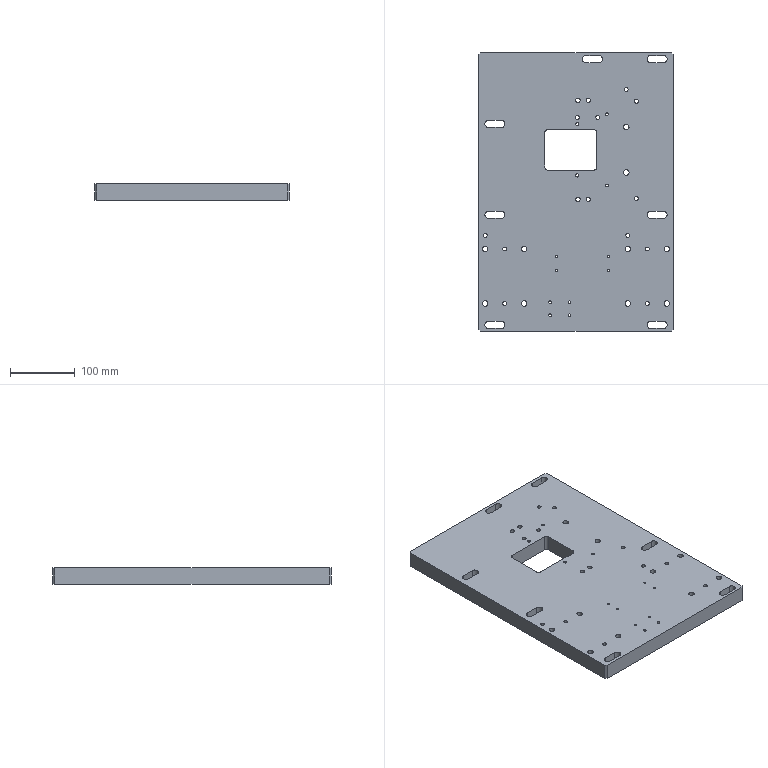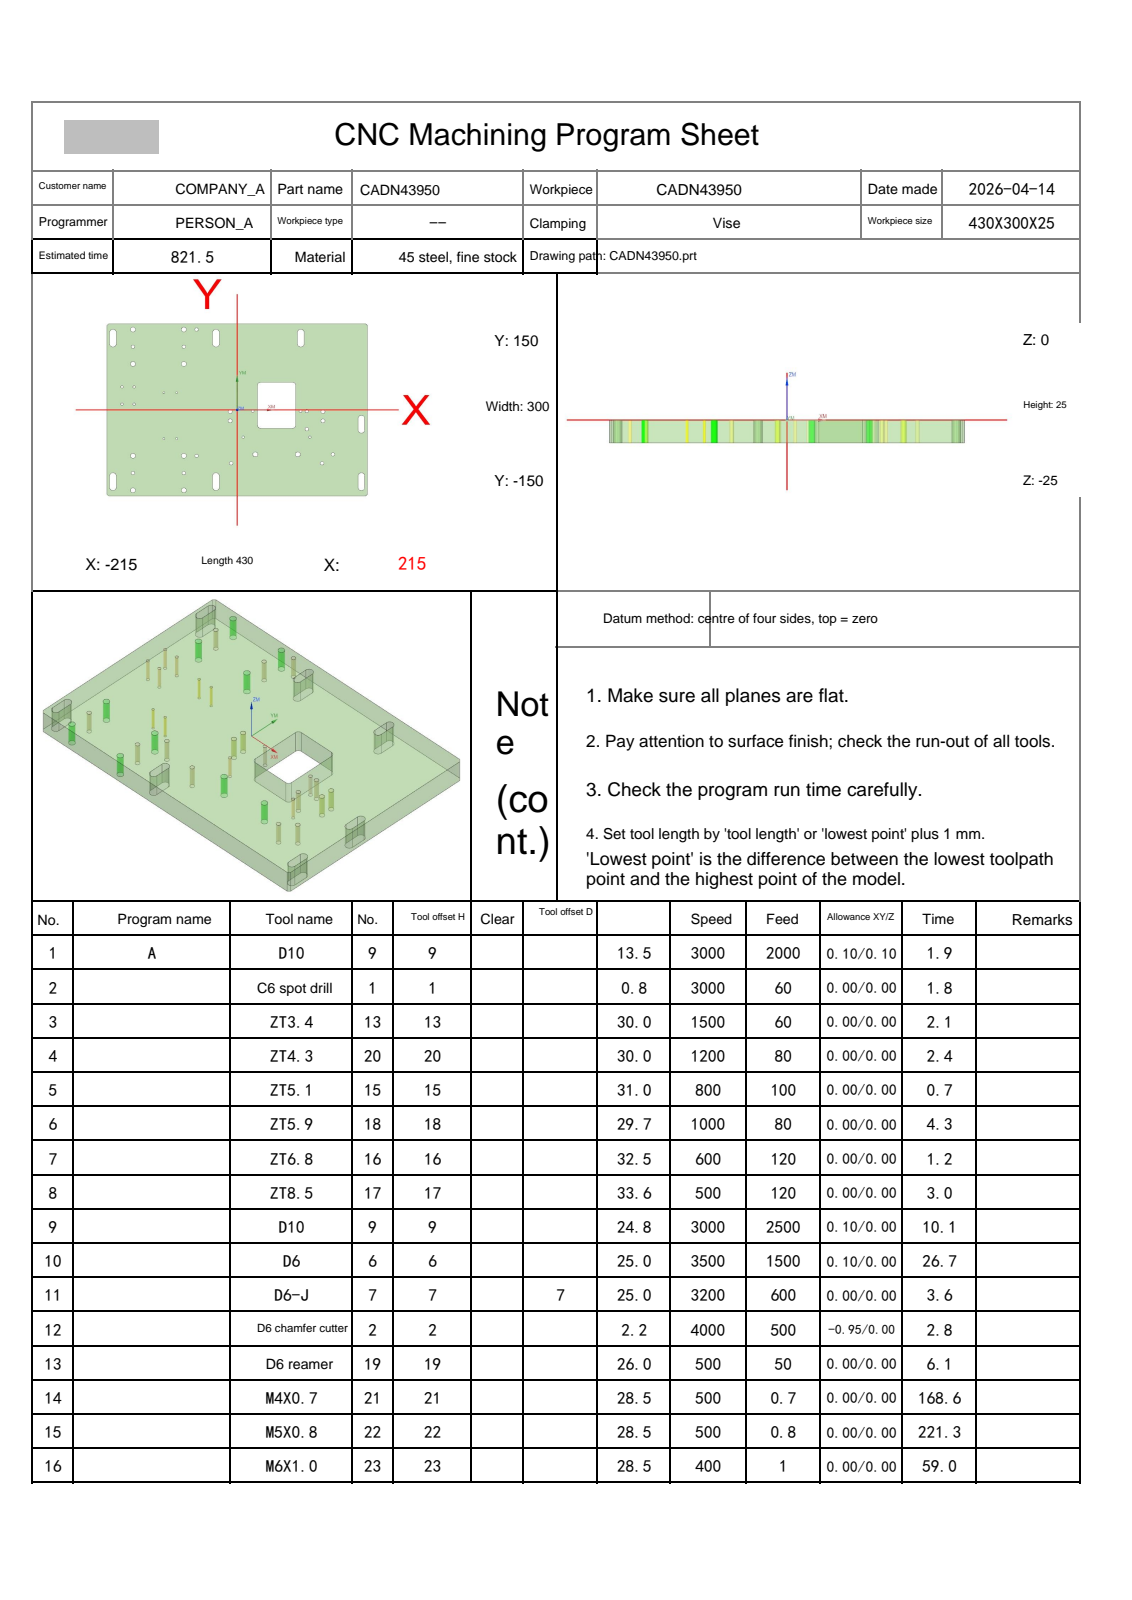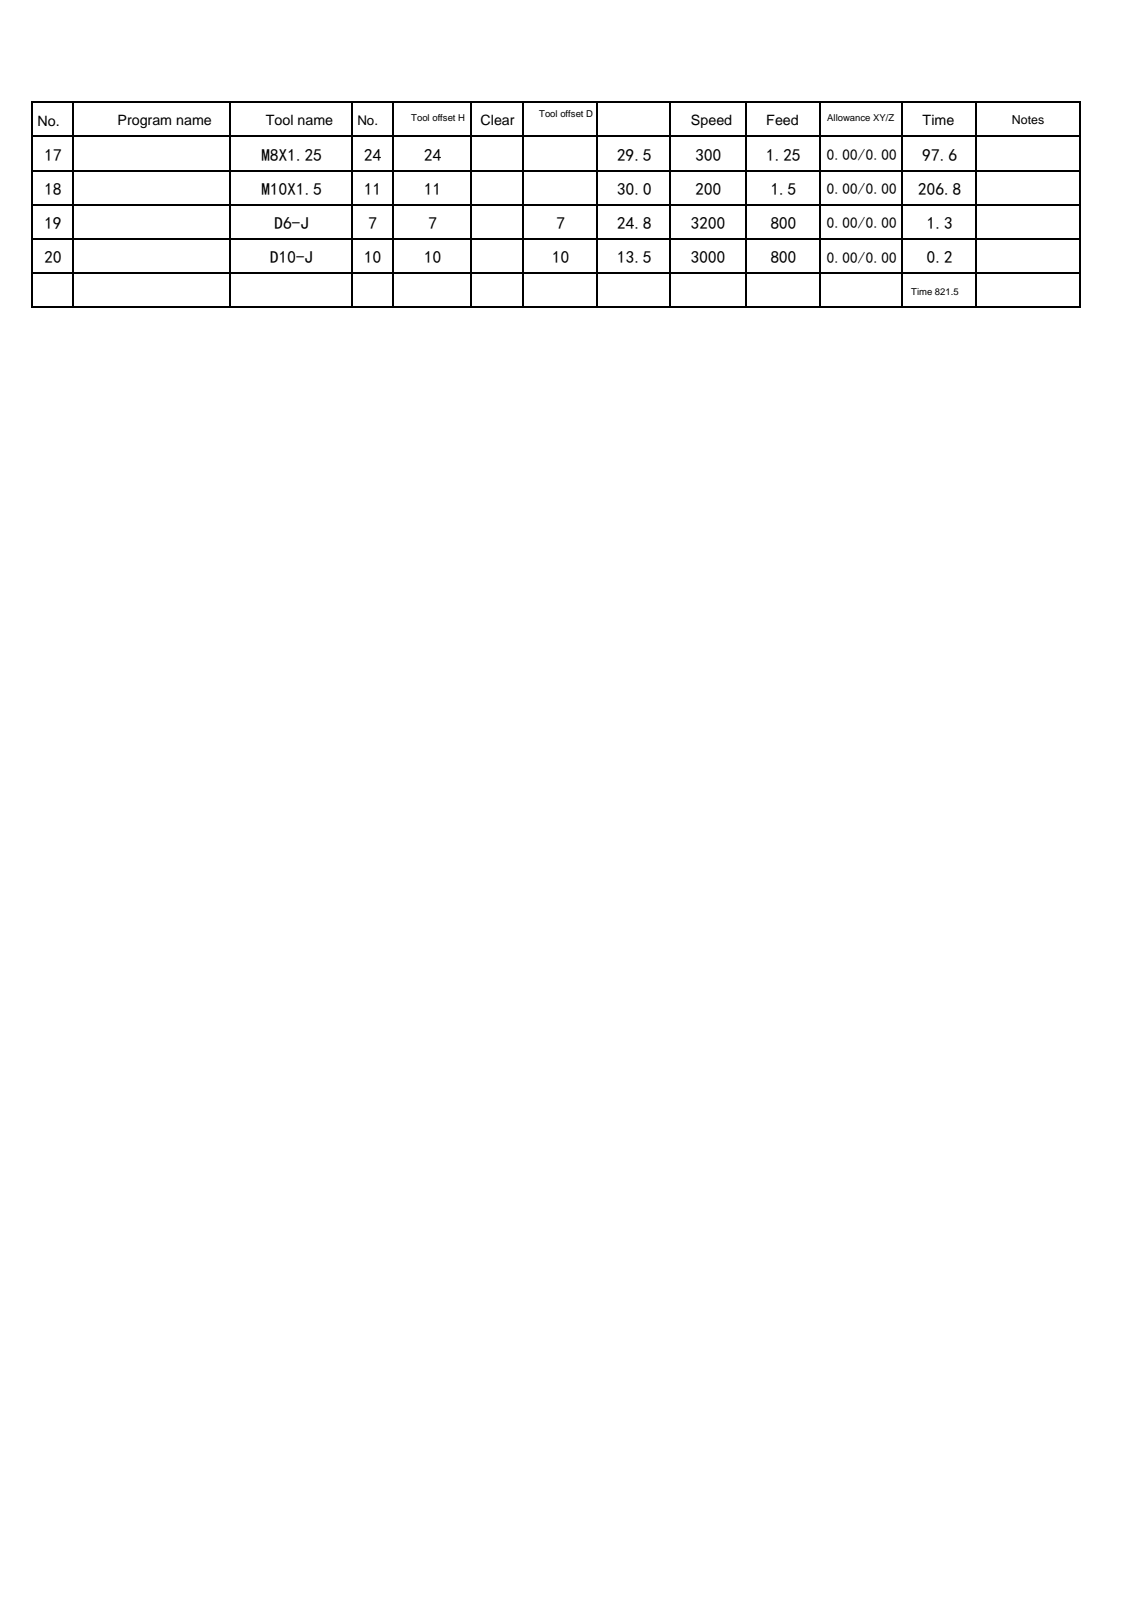NC program | NX | posted by the shop | part box 300 x 430 x 25 mm
Lines 1 to 1268 of 7024:
%
O0001
(Machine time: 1552.86 MIN)
(===Total Tool:18===)
(T9=D10     D=10.  R=0.   D-  H09 Z=-24.8 )
(T1=C6 spot drill D=6. R=0. D- H01 Z=-0.8  )
(T13=ZT3.4  D=3.4  DR_a=118 D-  H13 Z=-30.  )
(T20=ZT4.3  D=4.3  DR_a=118 D-  H20 Z=-30.  )
(T15=ZT5.1  D=5.1  DR_a=118 D-  H15 Z=-31.  )
(T18=ZT5.9  D=5.9  DR_a=120 D-  H18 Z=-29.7 )
(T16=ZT6.8  D=6.8  DR_a=118 D-  H16 Z=-32.54)
(T17=ZT8.5  D=8.5  DR_a=118 D-  H17 Z=-33.55)
(T6=D6      D=6.   R=0.   D-  H06 Z=-25.  )
(T7=D6-J    D=6.   R=0.   D7  H07 Z=-25.  )
(T2=D6 chamfer cutter D=6. R=0. D- H02 Z=-2.2  )
(T19=D6 reamer D=6. DR_a=180 D- H19 Z=-26.  )
(T21=M4X0.7 D=3.3  DR_a=180 D-  H21 Z=-28.5 )
(T22=M5X0.8 D=4.2  DR_a=180 D-  H22 Z=-28.5 )
(T23=M6X1.0 D=5.   DR_a=180 D-  H23 Z=-28.5 )
(T24=M8X1.25 D=6.8  DR_a=180 D-  H24 Z=-29.5 )
(T11=M10X1.5 D=8.5  DR_a=180 D-  H11 Z=-30.  )
(T10=D10-J  D=10.  R=0.   D10 H10 Z=-13.5 )
G80 G90 G17 G49 G40
G91 G28 Z0
M01
N1 T09 M06
(D10  D=10. R=0. H=09 ce=0.10 di=0.10)
G00 G90 G54 X-225.1 Y144.112 M03 S3000
G43 H09 Z20.
M08
Z-.346
G01 X-218.606 Y150.606 F2000.
X-215.606 Y153.606
X-209.112 Y160.1
G00 Z-.692
G01 X-215.606 Y153.606
X-218.606 Y150.606
X-225.1 Y144.112
G00 Z-1.038
G01 X-218.606 Y150.606
X-215.606 Y153.606
X-209.112 Y160.1
G00 Z-1.385
G01 X-215.606 Y153.606
X-218.606 Y150.606
X-225.1 Y144.112
G00 Z-1.731
G01 X-218.606 Y150.606
X-215.606 Y153.606
X-209.112 Y160.1
G00 Z-2.077
G01 X-215.606 Y153.606
X-218.606 Y150.606
X-225.1 Y144.112
G00 Z-2.423
G01 X-218.606 Y150.606
X-215.606 Y153.606
X-209.112 Y160.1
G00 Z-2.769
G01 X-215.606 Y153.606
X-218.606 Y150.606
X-225.1 Y144.112
G00 Z-3.115
G01 X-218.606 Y150.606
X-215.606 Y153.606
X-209.112 Y160.1
G00 Z-3.462
G01 X-215.606 Y153.606
X-218.606 Y150.606
X-225.1 Y144.112
G00 Z-3.808
G01 X-218.606 Y150.606
X-215.606 Y153.606
X-209.112 Y160.1
G00 Z-4.154
G01 X-215.606 Y153.606
X-218.606 Y150.606
X-225.1 Y144.112
G00 Z-4.5
G01 X-218.606 Y150.606
X-215.606 Y153.606
X-209.112 Y160.1
G00 Z-4.846
G01 X-215.606 Y153.606
X-218.606 Y150.606
X-225.1 Y144.112
G00 Z-5.192
G01 X-218.606 Y150.606
X-215.606 Y153.606
X-209.112 Y160.1
G00 Z-5.538
G01 X-215.606 Y153.606
X-218.606 Y150.606
X-225.1 Y144.112
G00 Z-5.885
G01 X-218.606 Y150.606
X-215.606 Y153.606
X-209.112 Y160.1
G00 Z-6.231
G01 X-215.606 Y153.606
X-218.606 Y150.606
X-225.1 Y144.112
G00 Z-6.577
G01 X-218.606 Y150.606
X-215.606 Y153.606
X-209.112 Y160.1
G00 Z-6.923
G01 X-215.606 Y153.606
X-218.606 Y150.606
X-225.1 Y144.112
G00 Z-7.269
G01 X-218.606 Y150.606
X-215.606 Y153.606
X-209.112 Y160.1
G00 Z-7.615
G01 X-215.606 Y153.606
X-218.606 Y150.606
X-225.1 Y144.112
G00 Z-7.962
G01 X-218.606 Y150.606
X-215.606 Y153.606
X-209.112 Y160.1
G00 Z-8.308
G01 X-215.606 Y153.606
X-218.606 Y150.606
X-225.1 Y144.112
G00 Z-8.654
G01 X-218.606 Y150.606
X-215.606 Y153.606
X-209.112 Y160.1
G00 Z-9.
G01 X-215.606 Y153.606
X-218.606 Y150.606
X-225.1 Y144.112
G00 Z-9.346
G01 X-218.606 Y150.606
X-215.606 Y153.606
X-209.112 Y160.1
G00 Z-9.692
G01 X-215.606 Y153.606
X-218.606 Y150.606
X-225.1 Y144.112
G00 Z-10.038
G01 X-218.606 Y150.606
X-215.606 Y153.606
X-209.112 Y160.1
G00 Z-10.385
G01 X-215.606 Y153.606
X-218.606 Y150.606
X-225.1 Y144.112
G00 Z-10.731
G01 X-218.606 Y150.606
X-215.606 Y153.606
X-209.112 Y160.1
G00 Z-11.077
G01 X-215.606 Y153.606
X-218.606 Y150.606
X-225.1 Y144.112
G00 Z-11.423
G01 X-218.606 Y150.606
X-215.606 Y153.606
X-209.112 Y160.1
G00 Z-11.769
G01 X-215.606 Y153.606
X-218.606 Y150.606
X-225.1 Y144.112
G00 Z-12.115
G01 X-218.606 Y150.606
X-215.606 Y153.606
X-209.112 Y160.1
G00 Z-12.462
G01 X-215.606 Y153.606
X-218.606 Y150.606
X-225.1 Y144.112
G00 Z-12.808
G01 X-218.606 Y150.606
X-215.606 Y153.606
X-209.112 Y160.1
G00 Z-13.154
G01 X-215.606 Y153.606
X-218.606 Y150.606
X-225.1 Y144.112
G00 Z-13.5
G01 X-218.606 Y150.606
X-215.606 Y153.606
X-209.112 Y160.1
G00 Z20.
Y-160.1
Z-.346
G01 X-215.606 Y-153.606
X-218.606 Y-150.606
X-225.1 Y-144.112
G00 Z-.692
G01 X-218.606 Y-150.606
X-215.606 Y-153.606
X-209.112 Y-160.1
G00 Z-1.038
G01 X-215.606 Y-153.606
X-218.606 Y-150.606
X-225.1 Y-144.112
G00 Z-1.385
G01 X-218.606 Y-150.606
X-215.606 Y-153.606
X-209.112 Y-160.1
G00 Z-1.731
G01 X-215.606 Y-153.606
X-218.606 Y-150.606
X-225.1 Y-144.112
G00 Z-2.077
G01 X-218.606 Y-150.606
X-215.606 Y-153.606
X-209.112 Y-160.1
G00 Z-2.423
G01 X-215.606 Y-153.606
X-218.606 Y-150.606
X-225.1 Y-144.112
G00 Z-2.769
G01 X-218.606 Y-150.606
X-215.606 Y-153.606
X-209.112 Y-160.1
G00 Z-3.115
G01 X-215.606 Y-153.606
X-218.606 Y-150.606
X-225.1 Y-144.112
G00 Z-3.462
G01 X-218.606 Y-150.606
X-215.606 Y-153.606
X-209.112 Y-160.1
G00 Z-3.808
G01 X-215.606 Y-153.606
X-218.606 Y-150.606
X-225.1 Y-144.112
G00 Z-4.154
G01 X-218.606 Y-150.606
X-215.606 Y-153.606
X-209.112 Y-160.1
G00 Z-4.5
G01 X-215.606 Y-153.606
X-218.606 Y-150.606
X-225.1 Y-144.112
G00 Z-4.846
G01 X-218.606 Y-150.606
X-215.606 Y-153.606
X-209.112 Y-160.1
G00 Z-5.192
G01 X-215.606 Y-153.606
X-218.606 Y-150.606
X-225.1 Y-144.112
G00 Z-5.538
G01 X-218.606 Y-150.606
X-215.606 Y-153.606
X-209.112 Y-160.1
G00 Z-5.885
G01 X-215.606 Y-153.606
X-218.606 Y-150.606
X-225.1 Y-144.112
G00 Z-6.231
G01 X-218.606 Y-150.606
X-215.606 Y-153.606
X-209.112 Y-160.1
G00 Z-6.577
G01 X-215.606 Y-153.606
X-218.606 Y-150.606
X-225.1 Y-144.112
G00 Z-6.923
G01 X-218.606 Y-150.606
X-215.606 Y-153.606
X-209.112 Y-160.1
G00 Z-7.269
G01 X-215.606 Y-153.606
X-218.606 Y-150.606
X-225.1 Y-144.112
G00 Z-7.615
G01 X-218.606 Y-150.606
X-215.606 Y-153.606
X-209.112 Y-160.1
G00 Z-7.962
G01 X-215.606 Y-153.606
X-218.606 Y-150.606
X-225.1 Y-144.112
G00 Z-8.308
G01 X-218.606 Y-150.606
X-215.606 Y-153.606
X-209.112 Y-160.1
G00 Z-8.654
G01 X-215.606 Y-153.606
X-218.606 Y-150.606
X-225.1 Y-144.112
G00 Z-9.
G01 X-218.606 Y-150.606
X-215.606 Y-153.606
X-209.112 Y-160.1
G00 Z-9.346
G01 X-215.606 Y-153.606
X-218.606 Y-150.606
X-225.1 Y-144.112
G00 Z-9.692
G01 X-218.606 Y-150.606
X-215.606 Y-153.606
X-209.112 Y-160.1
G00 Z-10.038
G01 X-215.606 Y-153.606
X-218.606 Y-150.606
X-225.1 Y-144.112
G00 Z-10.385
G01 X-218.606 Y-150.606
X-215.606 Y-153.606
X-209.112 Y-160.1
G00 Z-10.731
G01 X-215.606 Y-153.606
X-218.606 Y-150.606
X-225.1 Y-144.112
G00 Z-11.077
G01 X-218.606 Y-150.606
X-215.606 Y-153.606
X-209.112 Y-160.1
G00 Z-11.423
G01 X-215.606 Y-153.606
X-218.606 Y-150.606
X-225.1 Y-144.112
G00 Z-11.769
G01 X-218.606 Y-150.606
X-215.606 Y-153.606
X-209.112 Y-160.1
G00 Z-12.115
G01 X-215.606 Y-153.606
X-218.606 Y-150.606
X-225.1 Y-144.112
G00 Z-12.462
G01 X-218.606 Y-150.606
X-215.606 Y-153.606
X-209.112 Y-160.1
G00 Z-12.808
G01 X-215.606 Y-153.606
X-218.606 Y-150.606
X-225.1 Y-144.112
G00 Z-13.154
G01 X-218.606 Y-150.606
X-215.606 Y-153.606
X-209.112 Y-160.1
G00 Z-13.5
G01 X-215.606 Y-153.606
X-218.606 Y-150.606
X-225.1 Y-144.112
G00 Z20.
X225.1
Z-.346
G01 X218.606 Y-150.606
X215.606 Y-153.606
X209.112 Y-160.1
G00 Z-.692
G01 X215.606 Y-153.606
X218.606 Y-150.606
X225.1 Y-144.112
G00 Z-1.038
G01 X218.606 Y-150.606
X215.606 Y-153.606
X209.112 Y-160.1
G00 Z-1.385
G01 X215.606 Y-153.606
X218.606 Y-150.606
X225.1 Y-144.112
G00 Z-1.731
G01 X218.606 Y-150.606
X215.606 Y-153.606
X209.112 Y-160.1
G00 Z-2.077
G01 X215.606 Y-153.606
X218.606 Y-150.606
X225.1 Y-144.112
G00 Z-2.423
G01 X218.606 Y-150.606
X215.606 Y-153.606
X209.112 Y-160.1
G00 Z-2.769
G01 X215.606 Y-153.606
X218.606 Y-150.606
X225.1 Y-144.112
G00 Z-3.115
G01 X218.606 Y-150.606
X215.606 Y-153.606
X209.112 Y-160.1
G00 Z-3.462
G01 X215.606 Y-153.606
X218.606 Y-150.606
X225.1 Y-144.112
G00 Z-3.808
G01 X218.606 Y-150.606
X215.606 Y-153.606
X209.112 Y-160.1
G00 Z-4.154
G01 X215.606 Y-153.606
X218.606 Y-150.606
X225.1 Y-144.112
G00 Z-4.5
G01 X218.606 Y-150.606
X215.606 Y-153.606
X209.112 Y-160.1
G00 Z-4.846
G01 X215.606 Y-153.606
X218.606 Y-150.606
X225.1 Y-144.112
G00 Z-5.192
G01 X218.606 Y-150.606
X215.606 Y-153.606
X209.112 Y-160.1
G00 Z-5.538
G01 X215.606 Y-153.606
X218.606 Y-150.606
X225.1 Y-144.112
G00 Z-5.885
G01 X218.606 Y-150.606
X215.606 Y-153.606
X209.112 Y-160.1
G00 Z-6.231
G01 X215.606 Y-153.606
X218.606 Y-150.606
X225.1 Y-144.112
G00 Z-6.577
G01 X218.606 Y-150.606
X215.606 Y-153.606
X209.112 Y-160.1
G00 Z-6.923
G01 X215.606 Y-153.606
X218.606 Y-150.606
X225.1 Y-144.112
G00 Z-7.269
G01 X218.606 Y-150.606
X215.606 Y-153.606
X209.112 Y-160.1
G00 Z-7.615
G01 X215.606 Y-153.606
X218.606 Y-150.606
X225.1 Y-144.112
G00 Z-7.962
G01 X218.606 Y-150.606
X215.606 Y-153.606
X209.112 Y-160.1
G00 Z-8.308
G01 X215.606 Y-153.606
X218.606 Y-150.606
X225.1 Y-144.112
G00 Z-8.654
G01 X218.606 Y-150.606
X215.606 Y-153.606
X209.112 Y-160.1
G00 Z-9.
G01 X215.606 Y-153.606
X218.606 Y-150.606
X225.1 Y-144.112
G00 Z-9.346
G01 X218.606 Y-150.606
X215.606 Y-153.606
X209.112 Y-160.1
G00 Z-9.692
G01 X215.606 Y-153.606
X218.606 Y-150.606
X225.1 Y-144.112
G00 Z-10.038
G01 X218.606 Y-150.606
X215.606 Y-153.606
X209.112 Y-160.1
G00 Z-10.385
G01 X215.606 Y-153.606
X218.606 Y-150.606
X225.1 Y-144.112
G00 Z-10.731
G01 X218.606 Y-150.606
X215.606 Y-153.606
X209.112 Y-160.1
G00 Z-11.077
G01 X215.606 Y-153.606
X218.606 Y-150.606
X225.1 Y-144.112
G00 Z-11.423
G01 X218.606 Y-150.606
X215.606 Y-153.606
X209.112 Y-160.1
G00 Z-11.769
G01 X215.606 Y-153.606
X218.606 Y-150.606
X225.1 Y-144.112
G00 Z-12.115
G01 X218.606 Y-150.606
X215.606 Y-153.606
X209.112 Y-160.1
G00 Z-12.462
G01 X215.606 Y-153.606
X218.606 Y-150.606
X225.1 Y-144.112
G00 Z-12.808
G01 X218.606 Y-150.606
X215.606 Y-153.606
X209.112 Y-160.1
G00 Z-13.154
G01 X215.606 Y-153.606
X218.606 Y-150.606
X225.1 Y-144.112
G00 Z-13.5
G01 X218.606 Y-150.606
X215.606 Y-153.606
X209.112 Y-160.1
G00 Z20.
Y160.1
Z-.346
G01 X215.606 Y153.606
X218.606 Y150.606
X225.1 Y144.112
G00 Z-.692
G01 X218.606 Y150.606
X215.606 Y153.606
X209.112 Y160.1
G00 Z-1.038
G01 X215.606 Y153.606
X218.606 Y150.606
X225.1 Y144.112
G00 Z-1.385
G01 X218.606 Y150.606
X215.606 Y153.606
X209.112 Y160.1
G00 Z-1.731
G01 X215.606 Y153.606
X218.606 Y150.606
X225.1 Y144.112
G00 Z-2.077
G01 X218.606 Y150.606
X215.606 Y153.606
X209.112 Y160.1
G00 Z-2.423
G01 X215.606 Y153.606
X218.606 Y150.606
X225.1 Y144.112
G00 Z-2.769
G01 X218.606 Y150.606
X215.606 Y153.606
X209.112 Y160.1
G00 Z-3.115
G01 X215.606 Y153.606
X218.606 Y150.606
X225.1 Y144.112
G00 Z-3.462
G01 X218.606 Y150.606
X215.606 Y153.606
X209.112 Y160.1
G00 Z-3.808
G01 X215.606 Y153.606
X218.606 Y150.606
X225.1 Y144.112
G00 Z-4.154
G01 X218.606 Y150.606
X215.606 Y153.606
X209.112 Y160.1
G00 Z-4.5
G01 X215.606 Y153.606
X218.606 Y150.606
X225.1 Y144.112
G00 Z-4.846
G01 X218.606 Y150.606
X215.606 Y153.606
X209.112 Y160.1
G00 Z-5.192
G01 X215.606 Y153.606
X218.606 Y150.606
X225.1 Y144.112
G00 Z-5.538
G01 X218.606 Y150.606
X215.606 Y153.606
X209.112 Y160.1
G00 Z-5.885
G01 X215.606 Y153.606
X218.606 Y150.606
X225.1 Y144.112
G00 Z-6.231
G01 X218.606 Y150.606
X215.606 Y153.606
X209.112 Y160.1
G00 Z-6.577
G01 X215.606 Y153.606
X218.606 Y150.606
X225.1 Y144.112
G00 Z-6.923
G01 X218.606 Y150.606
X215.606 Y153.606
X209.112 Y160.1
G00 Z-7.269
G01 X215.606 Y153.606
X218.606 Y150.606
X225.1 Y144.112
G00 Z-7.615
G01 X218.606 Y150.606
X215.606 Y153.606
X209.112 Y160.1
G00 Z-7.962
G01 X215.606 Y153.606
X218.606 Y150.606
X225.1 Y144.112
G00 Z-8.308
G01 X218.606 Y150.606
X215.606 Y153.606
X209.112 Y160.1
G00 Z-8.654
G01 X215.606 Y153.606
X218.606 Y150.606
X225.1 Y144.112
G00 Z-9.
G01 X218.606 Y150.606
X215.606 Y153.606
X209.112 Y160.1
G00 Z-9.346
G01 X215.606 Y153.606
X218.606 Y150.606
X225.1 Y144.112
G00 Z-9.692
G01 X218.606 Y150.606
X215.606 Y153.606
X209.112 Y160.1
G00 Z-10.038
G01 X215.606 Y153.606
X218.606 Y150.606
X225.1 Y144.112
G00 Z-10.385
G01 X218.606 Y150.606
X215.606 Y153.606
X209.112 Y160.1
G00 Z-10.731
G01 X215.606 Y153.606
X218.606 Y150.606
X225.1 Y144.112
G00 Z-11.077
G01 X218.606 Y150.606
X215.606 Y153.606
X209.112 Y160.1
G00 Z-11.423
G01 X215.606 Y153.606
X218.606 Y150.606
X225.1 Y144.112
G00 Z-11.769
G01 X218.606 Y150.606
X215.606 Y153.606
X209.112 Y160.1
G00 Z-12.115
G01 X215.606 Y153.606
X218.606 Y150.606
X225.1 Y144.112
G00 Z-12.462
G01 X218.606 Y150.606
X215.606 Y153.606
X209.112 Y160.1
G00 Z-12.808
G01 X215.606 Y153.606
X218.606 Y150.606
X225.1 Y144.112
G00 Z-13.154
G01 X218.606 Y150.606
X215.606 Y153.606
X209.112 Y160.1
G00 Z-13.5
G01 X215.606 Y153.606
X218.606 Y150.606
X225.1 Y144.112
G00 Z20.
G91 G28 Z0.0
M05
M09
G91 G28 Z0.0
M01
N2 T01 M06
(C6 spot drill D=6. R=0. H=01 ce=0.00 di=0.10)
G00 G90 G54 X158. Y-77.5 M03 S3000
G43 H01 Z20.
M08
G98 G81 X158. Y-77.5 Z-.8 R1. F60.
X140. Y-93.
X100. Y-77.5
X120. Y-47.5
X115. Y-33.5
X141.5 Y-19.
Y-3.
X115. Y-2.
X104.5
X25.5
X-11.5 Y-3.
Y-19.
X10. Y-47.5
X30. Y-77.5
X-10. Y-93.
X-67. Y-80.
X-88.
Y-110.
Y-140.
X-172.
Y-110.
Y-80.
X-121. Y-50.
X-100.
Y30.
X-121.
X-170. Y10.
X-190.
Y40.
X-170.
X-172. Y80.
Y110.
Y140.
X-88.
X-67.
X-88. Y110.
Y80.
X-205. Y135.
Y115.
Y-115.
Y-135.
X-35. Y-115.
Y-135.
X205. Y-115.
Y-135.
Y-15.
Y-35.
X105. Y135.
Y115.
X-35. Y135.
Y115.
G80
G00 Z20.
G91 G28 Z0.0
M05
M09
G91 G28 Z0.0
M01
N3 T13 M06
(ZT3.4 D=3.4 DR_a=118 H=13)
G00 G90 G54 X-121. Y-50. M03 S1500
G43 H13 Z20.
M08
G98 G83 X-121. Y-50. Z-30. R1. F60. Q1.
X-100.
Y30.
X-121.
G80
G00 Z20.
G91 G28 Z0.0
M05
M09
G91 G28 Z0.0
M01
N4 T20 M06
(ZT4.3 D=4.3 DR_a=118 H=20)
G00 G90 G54 X-170. Y40. M03 S1200
G43 H20 Z20.
M08
G98 G83 X-170. Y40. Z-30. R1. F80. Q1.5
X-190.
Y10.
X-170.
X10. Y-47.5
X120.
G80
G00 Z20.
G91 G28 Z0.0
M05
M09
G91 G28 Z0.0
M01
N5 T15 M06
(ZT5.1 D=5.1 DR_a=118 H=15)
G00 G90 G54 X25.5 Y-2. M03 S800
G43 H15 Z20.
M08
G98 G83 X25.5 Y-2. Z-31. R1. F100. Q2.
X104.5
G80
G00 Z20.
G91 G28 Z0.0
M05
M09
G91 G28 Z0.0
M01
N6 T18 M06
(ZT5.9 D=5.9 DR_a=120 H=18)
G00 G90 G54 X-67. Y140. M03 S1000
G43 H18 Z20.
M08
G98 G83 X-67. Y140. Z-29.703 R1. F80. Q1.
X-88. Y110.
X-172.
Y-110.
X-88.
X-67. Y-80.
X-10. Y-93.
X140.
X158. Y-77.5
X115. Y-33.5
Y-2.
G80
G00 Z20.
G91 G28 Z0.0
M05
M09
G91 G28 Z0.0
M01
N7 T16 M06
(ZT6.8 D=6.8 DR_a=118 H=16)
G00 G90 G54 X141.5 Y-3. M03 S600
G43 H16 Z20.
M08
G98 G83 X141.5 Y-3. Z-32.543 R1. F120. Q2.
Y-19.
X-11.5
Y-3.
G80
G00 Z20.
G91 G28 Z0.0
M05
M09
G91 G28 Z0.0
M01
N8 T17 M06
(ZT8.5 D=8.5 DR_a=118 H=17)
G00 G90 G54 X-88. Y80. M03 S500
G43 H17 Z20.
M08
G98 G83 X-88. Y80. Z-33.554 R1. F120. Q2.
Y140.
X-172.
Y80.
Y-80.
Y-140.
X-88.
Y-80.
X30. Y-77.5
X100.
G80
G00 Z20.
G91 G28 Z0.0
M05
M09
G91 G28 Z0.0
M01
N9 T09 M06
(D10  D=10. R=0. H=09 ce=0.10 di=0.00)
G00 G90 G54 X91.4 Y8. M03 S3000
G43 H09 Z20.
M08
Z.5
G01 Y42.9 Z.465 F2500.
X38.6 Z.411
Y-26.9 Z.341
X91.4 Z.287
Y42.9 Z.217
X38.6 Z.163
Y-26.9 Z.093
X91.4 Z.039
Y42.9 Z-.031
X38.6 Z-.085
Y-26.9 Z-.155
X91.4 Z-.209
Y42.9 Z-.279
X38.6 Z-.333
Y-26.9 Z-.403
X91.4 Z-.457
Y42.9 Z-.527
X38.6 Z-.581
Y-26.9 Z-.651
X91.4 Z-.705
Y42.9 Z-.776
X38.6 Z-.829
Y-26.9 Z-.9
X91.4 Z-.953
Y42.9 Z-1.024
X38.6 Z-1.077
Y-26.9 Z-1.148
X91.4 Z-1.201
Y42.9 Z-1.272
X38.6 Z-1.325
Y-26.9 Z-1.396
X91.4 Z-1.449
Y42.9 Z-1.52
X38.6 Z-1.573
Y-26.9 Z-1.644
X91.4 Z-1.697
Y42.9 Z-1.768
X38.6 Z-1.821
Y-26.9 Z-1.892
X91.4 Z-1.945
Y42.9 Z-2.016
X38.6 Z-2.069
Y-26.9 Z-2.14
X91.4 Z-2.193
Y42.9 Z-2.264
X38.6 Z-2.317
Y-26.9 Z-2.388
X91.4 Z-2.441
Y42.9 Z-2.512
X38.6 Z-2.565
Y-26.9 Z-2.636
X91.4 Z-2.689
Y42.9 Z-2.76
X38.6 Z-2.813
Y-26.9 Z-2.884
X91.4 Z-2.937
Y42.9 Z-3.008
X38.6 Z-3.061
Y-26.9 Z-3.132
X91.4 Z-3.185
Y42.9 Z-3.256
X38.6 Z-3.309
Y-26.9 Z-3.38
X91.4 Z-3.433
Y42.9 Z-3.504
X38.6 Z-3.557
Y-26.9 Z-3.628
X91.4 Z-3.681
Y42.9 Z-3.752
X38.6 Z-3.805
Y-26.9 Z-3.876
X91.4 Z-3.929
Y42.9 Z-4.
X38.6 Z-4.053
Y-26.9 Z-4.124
X91.4 Z-4.177
Y42.9 Z-4.248
X38.6 Z-4.301
Y-26.9 Z-4.372
X91.4 Z-4.425
Y42.9 Z-4.496
X38.6 Z-4.55
Y-26.9 Z-4.62
X91.4 Z-4.674
Y42.9 Z-4.744
X38.6 Z-4.798
Y-26.9 Z-4.868
X91.4 Z-4.922
Y42.9 Z-4.992
X38.6 Z-5.046
Y-26.9 Z-5.116
X91.4 Z-5.17
Y42.9 Z-5.24
X38.6 Z-5.294
Y-26.9 Z-5.364
X91.4 Z-5.418
Y42.9 Z-5.488
X38.6 Z-5.542
Y-26.9 Z-5.612
X91.4 Z-5.666
Y42.9 Z-5.736
X38.6 Z-5.79
Y-26.9 Z-5.86
X91.4 Z-5.914
Y42.9 Z-5.984
X38.6 Z-6.038
Y-26.9 Z-6.108
X91.4 Z-6.162
Y42.9 Z-6.232
X38.6 Z-6.286
Y-26.9 Z-6.356
X91.4 Z-6.41
Y42.9 Z-6.48
X38.6 Z-6.534
Y-26.9 Z-6.604
X91.4 Z-6.658
Y42.9 Z-6.728
X38.6 Z-6.782
Y-26.9 Z-6.852
X91.4 Z-6.906
Y42.9 Z-6.976
X38.6 Z-7.03
Y-26.9 Z-7.101
X91.4 Z-7.154
Y42.9 Z-7.225
X38.6 Z-7.278
Y-26.9 Z-7.349
X91.4 Z-7.402
Y42.9 Z-7.473
X38.6 Z-7.526
Y-26.9 Z-7.597
X91.4 Z-7.65
Y42.9 Z-7.721
X38.6 Z-7.774
Y-26.9 Z-7.845
X91.4 Z-7.898
Y42.9 Z-7.969
X38.6 Z-8.022
Y-26.9 Z-8.093
X91.4 Z-8.146
Y42.9 Z-8.217
X38.6 Z-8.27
Y-26.9 Z-8.341
X91.4 Z-8.394
Y42.9 Z-8.465
X38.6 Z-8.518
Y-26.9 Z-8.589
X91.4 Z-8.642
Y42.9 Z-8.713
X38.6 Z-8.766
Y-26.9 Z-8.837
X91.4 Z-8.89
Y42.9 Z-8.961
X38.6 Z-9.014
Y-26.9 Z-9.085
X91.4 Z-9.138
Y42.9 Z-9.209
X38.6 Z-9.262
Y-26.9 Z-9.333
X91.4 Z-9.386
Y42.9 Z-9.457
X38.6 Z-9.51
Y-26.9 Z-9.581
X91.4 Z-9.634
Y42.9 Z-9.705
X38.6 Z-9.758
Y-26.9 Z-9.829
X91.4 Z-9.882
Y42.9 Z-9.953
X38.6 Z-10.006
Y-26.9 Z-10.077
X91.4 Z-10.13
Y42.9 Z-10.201
X38.6 Z-10.254
Y-26.9 Z-10.325
X91.4 Z-10.378
Y42.9 Z-10.449
X38.6 Z-10.502
Y-26.9 Z-10.573
X91.4 Z-10.626
Y42.9 Z-10.697
X38.6 Z-10.75
Y-26.9 Z-10.821
X91.4 Z-10.875
Y42.9 Z-10.945
X38.6 Z-10.999
Y-26.9 Z-11.069
X91.4 Z-11.123
Y42.9 Z-11.193
X38.6 Z-11.247
Y-26.9 Z-11.317
X91.4 Z-11.371
Y42.9 Z-11.441
X38.6 Z-11.495
Y-26.9 Z-11.565
X91.4 Z-11.619
Y42.9 Z-11.689
X38.6 Z-11.743
Y-26.9 Z-11.813
X91.4 Z-11.867
Y42.9 Z-11.937
X38.6 Z-11.991
Y-26.9 Z-12.061
X91.4 Z-12.115
Y42.9 Z-12.185
X38.6 Z-12.239
Y-26.9 Z-12.309
X91.4 Z-12.363
Y42.9 Z-12.433
X38.6 Z-12.487
Y-26.9 Z-12.557
X91.4 Z-12.611
Y42.9 Z-12.681
X38.6 Z-12.735
Y-26.9 Z-12.805
X91.4 Z-12.859
Y42.9 Z-12.929
X38.6 Z-12.983
Y-26.9 Z-13.053
X91.4 Z-13.107
Y42.9 Z-13.177
X38.6 Z-13.231
Y-26.9 Z-13.301
X91.4 Z-13.355
Y42.9 Z-13.426
X38.6 Z-13.479
Y-26.9 Z-13.55
X91.4 Z-13.603
Y42.9 Z-13.674
X38.6 Z-13.727
Y-26.9 Z-13.798
X91.4 Z-13.851
Y42.9 Z-13.922
X38.6 Z-13.975
Y-26.9 Z-14.046
X91.4 Z-14.099
Y42.9 Z-14.17
X38.6 Z-14.223
Y-26.9 Z-14.294
X91.4 Z-14.347
Y42.9 Z-14.418
X38.6 Z-14.471
Y-26.9 Z-14.542
X91.4 Z-14.595
Y42.9 Z-14.666
X38.6 Z-14.719
Y-26.9 Z-14.79
X91.4 Z-14.843
Y42.9 Z-14.914
X38.6 Z-14.967
Y-26.9 Z-15.038
X91.4 Z-15.091
Y42.9 Z-15.162
X38.6 Z-15.215
Y-26.9 Z-15.286
X91.4 Z-15.339
Y42.9 Z-15.41
X38.6 Z-15.463
Y-26.9 Z-15.534
X91.4 Z-15.587
Y42.9 Z-15.658
X38.6 Z-15.711
Y-26.9 Z-15.782
X91.4 Z-15.835
Y42.9 Z-15.906
X38.6 Z-15.959
Y-26.9 Z-16.03
X91.4 Z-16.083
Y42.9 Z-16.154
X38.6 Z-16.207
Y-26.9 Z-16.278
X91.4 Z-16.331
Y42.9 Z-16.402
X38.6 Z-16.455
Y-26.9 Z-16.526
X91.4 Z-16.579
Y42.9 Z-16.65
X38.6 Z-16.703
Y-26.9 Z-16.774
X91.4 Z-16.827
Y42.9 Z-16.898
X38.6 Z-16.951
Y-26.9 Z-17.022
X91.4 Z-17.075
Y42.9 Z-17.146
X38.6 Z-17.2
Y-26.9 Z-17.27
X91.4 Z-17.324
Y42.9 Z-17.394
X38.6 Z-17.448
Y-26.9 Z-17.518
X91.4 Z-17.572
Y42.9 Z-17.642
X38.6 Z-17.696
Y-26.9 Z-17.766
X91.4 Z-17.82
Y42.9 Z-17.89
X38.6 Z-17.944
Y-26.9 Z-18.014
X91.4 Z-18.068
Y42.9 Z-18.138
X38.6 Z-18.192
Y-26.9 Z-18.262
X91.4 Z-18.316
Y42.9 Z-18.386
X38.6 Z-18.44
Y-26.9 Z-18.51
X91.4 Z-18.564
Y42.9 Z-18.634
X38.6 Z-18.688
Y-26.9 Z-18.758
X91.4 Z-18.812
Y42.9 Z-18.882
X38.6 Z-18.936
Y-26.9 Z-19.006
X91.4 Z-19.06
Y42.9 Z-19.13
X38.6 Z-19.184
Y-26.9 Z-19.254
X91.4 Z-19.308
Y42.9 Z-19.378
X38.6 Z-19.432
Y-26.9 Z-19.502
X91.4 Z-19.556
Y42.9 Z-19.626
X38.6 Z-19.68
Y-26.9 Z-19.751
X91.4 Z-19.804
Y42.9 Z-19.875
X38.6 Z-19.928
Y-26.9 Z-19.999
X91.4 Z-20.052
Y42.9 Z-20.123
X38.6 Z-20.176
Y-26.9 Z-20.247
X91.4 Z-20.3
Y42.9 Z-20.371
X38.6 Z-20.424
Y-26.9 Z-20.495
X91.4 Z-20.548
Y42.9 Z-20.619
X38.6 Z-20.672
Y-26.9 Z-20.743
X91.4 Z-20.796
Y42.9 Z-20.867
X38.6 Z-20.92
Y-26.9 Z-20.991
X91.4 Z-21.044
Y42.9 Z-21.115
X38.6 Z-21.168
Y-26.9 Z-21.239
X91.4 Z-21.292
Y42.9 Z-21.363
X38.6 Z-21.416
Y-26.9 Z-21.487
X91.4 Z-21.54
Y42.9 Z-21.611
X38.6 Z-21.664
Y-26.9 Z-21.735
X91.4 Z-21.788
Y42.9 Z-21.859
X38.6 Z-21.912
Y-26.9 Z-21.983
X91.4 Z-22.036
Y42.9 Z-22.107
X38.6 Z-22.16
Y-26.9 Z-22.231
X91.4 Z-22.284
Y42.9 Z-22.355
X38.6 Z-22.408
Y-26.9 Z-22.479
X91.4 Z-22.532
Y42.9 Z-22.603
X38.6 Z-22.656
Y-26.9 Z-22.727
X91.4 Z-22.78
Y42.9 Z-22.851
X38.6 Z-22.904
Y-26.9 Z-22.975
X91.4 Z-23.028
Y42.9 Z-23.099
X38.6 Z-23.152
Y-26.9 Z-23.223
X91.4 Z-23.276
Y42.9 Z-23.347
X38.6 Z-23.4
Y-26.9 Z-23.471
X91.4 Z-23.525
Y42.9 Z-23.595
X38.6 Z-23.649
Y-26.9 Z-23.719
X91.4 Z-23.773
Y42.9 Z-23.843
X38.6 Z-23.897
Y-26.9 Z-23.967
X91.4 Z-24.021
Y42.9 Z-24.091
X38.6 Z-24.145
Y-26.9 Z-24.215
X91.4 Z-24.269
Y42.9 Z-24.339
X38.6 Z-24.393
Y-26.9 Z-24.463
X91.4 Z-24.517
Y42.9 Z-24.587
X38.6 Z-24.641
Y-26.9 Z-24.711
X91.4 Z-24.765
Y8. Z-24.8
Y42.9
X38.6
Y-26.9
X91.4
Y8.
Y8.5
Z-23.8
G00 Z20.
G91 G28 Z0.0
M05
M09
G91 G28 Z0.0
M01